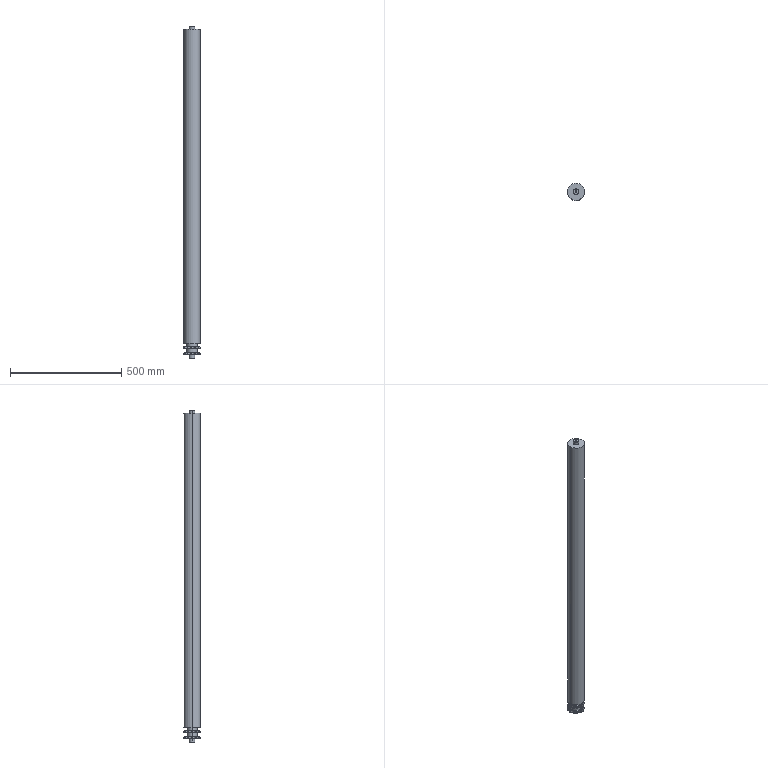Part | STEP file | 5分-13齿双排滚筒_GearTrax | 1 solid | 182 faces | box 76.009 x 76 x 1490 mm | volume 6520792 mm3 | cylinder 118 | torus 52 | plane 8 | cone 4 | commonest cylinder face diameters 36.576 x52 10.262 x26 76.019 x26 8.5 x4 25 x4 47 x4